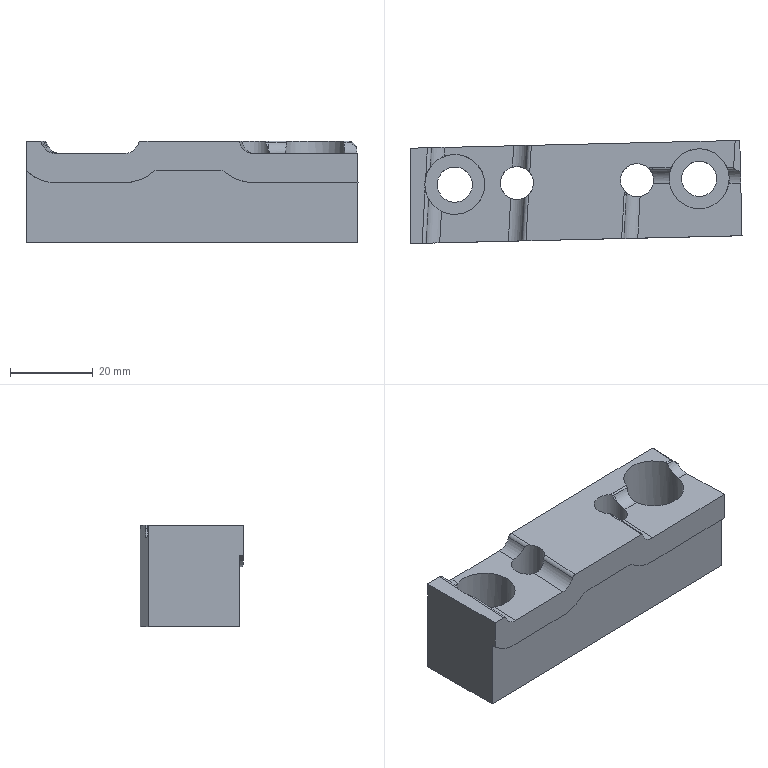Part | NX | features solid 2 | 1 solid | 38 faces | box 80.12 x 24.879 x 24.5 mm | volume 33585 mm3 | cylinder 20 | plane 13 | torus 4 | spline 1 | commonest cylinder face diameters 7 x7 2 x4 1 x3 8.001 x2 8.5 x2 14.5 x2